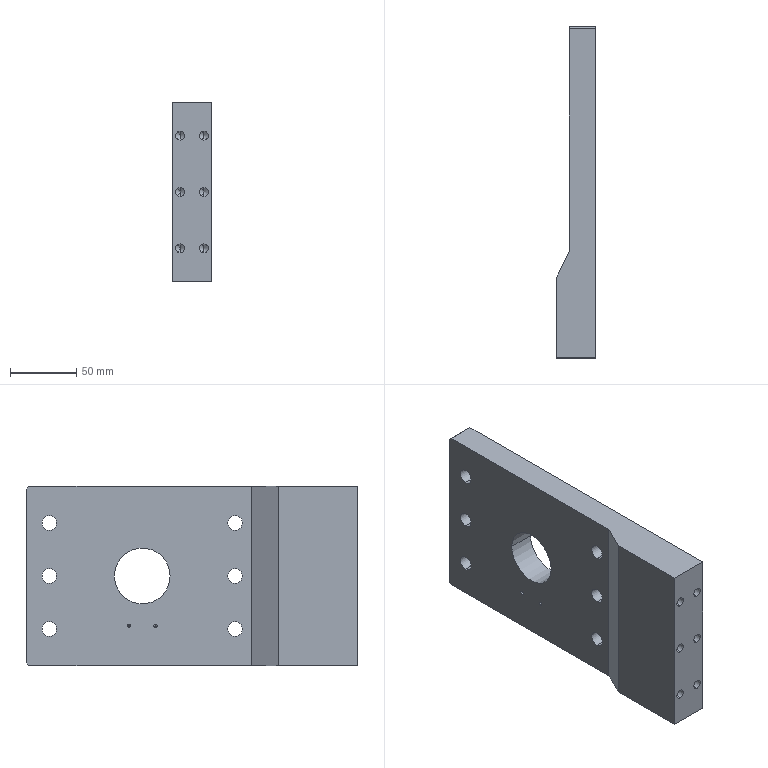Part | SolidWorks | features HoleWzd 4, Chamfer 1, Extrusion 1, ICE 1 | 1 solid | 82 faces | box 30 x 250 x 135 mm | volume 713772 mm3 | cylinder 46 | cone 20 | plane 16 | commonest cylinder face diameters 6.8 x16 11 x12 18 x12 2.5 x4 42 x2